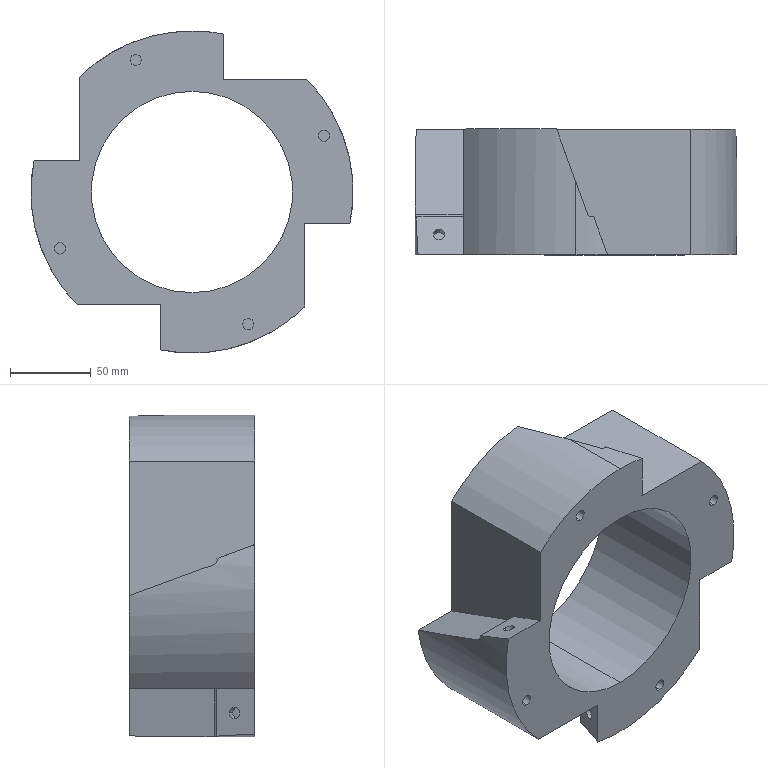Part | STEP file | Vibration plate 3-03_default | 1 solid | 49 faces | box 200 x 78 x 200 mm | volume 1058700 mm3 | cylinder 27 | plane 22 | commonest cylinder face diameters 7 x16 200 x5 6 x4 125 x2